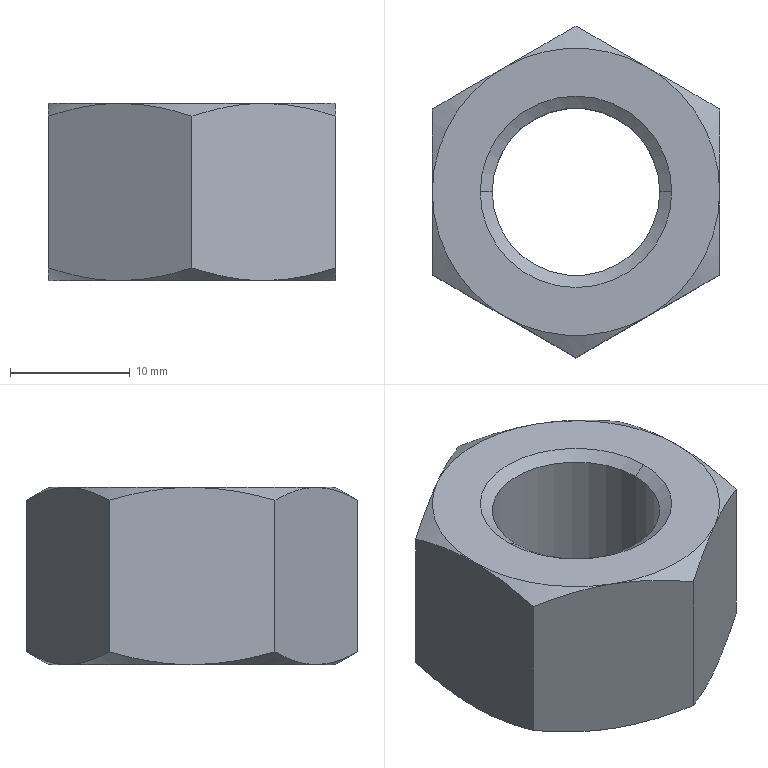Part | STEP file | hex nut style 1_am_B18.2.4.1M - Hex nut, Style 1,  M16 x 2 --D-N | 1 solid | 28 faces | box 24 x 27.713 x 14.8 mm | volume 5041 mm3 | cone 16 | plane 8 | cylinder 4 | commonest cylinder face diameters 14 x2 16 x2